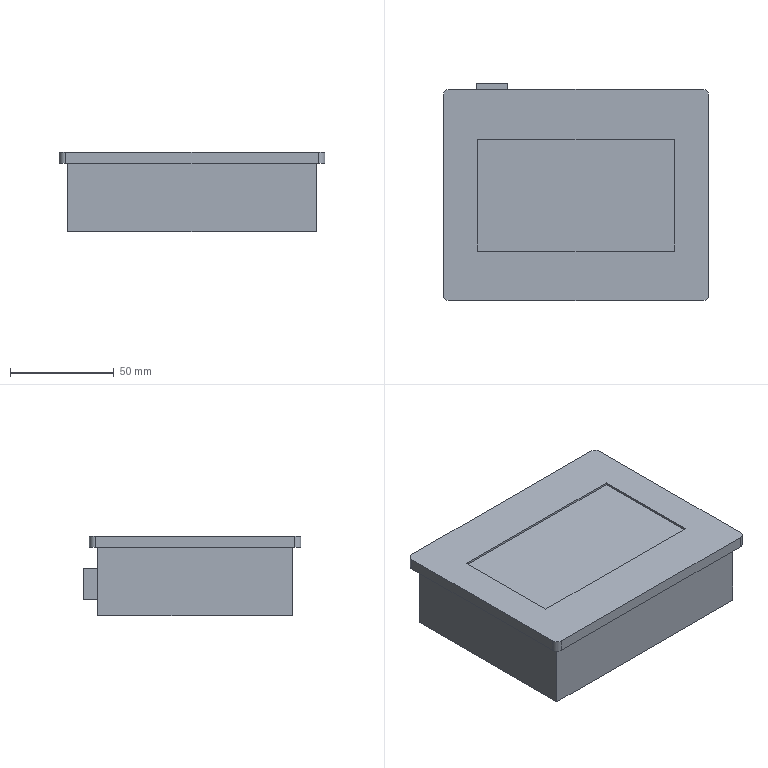Part | SolidWorks | features ICE 4, Extrusion 1, Fillet 1 | 2 solids | 31 faces | box 128 x 105 x 38.5 mm | volume 442026 mm3 | plane 27 | cylinder 4 | commonest cylinder face diameters 6 x4
STEP:
#1=CARTESIAN_POINT('',(-60.,47.,0.));
#2=VERTEX_POINT('',#1);
#3=CARTESIAN_POINT('',(60.,47.,0.));
#4=VERTEX_POINT('',#3);
#5=CARTESIAN_POINT('',(-60.,47.,0.));
#6=DIRECTION('',(1.,0.,0.));
#7=VECTOR('',#6,1000.);
#8=LINE('',#5,#7);
#9=EDGE_CURVE('',#2,#4,#8,.T.);
#10=ORIENTED_EDGE('',*,*,#9,.T.);
#11=CARTESIAN_POINT('',(60.,47.,-33.));
#12=VERTEX_POINT('',#11);
#13=CARTESIAN_POINT('',(60.,47.,-33.));
#14=DIRECTION('',(0.,0.,1.));
#15=VECTOR('',#14,1000.);
#16=LINE('',#13,#15);
#17=EDGE_CURVE('',#12,#4,#16,.T.);
#18=ORIENTED_EDGE('',*,*,#17,.F.);
#19=CARTESIAN_POINT('',(-60.,47.,-33.));
#20=VERTEX_POINT('',#19);
#21=CARTESIAN_POINT('',(-60.,47.,-33.));
#22=DIRECTION('',(1.,0.,0.));
#23=VECTOR('',#22,1000.);
#24=LINE('',#21,#23);
#25=EDGE_CURVE('',#20,#12,#24,.T.);
#26=ORIENTED_EDGE('',*,*,#25,.F.);
#27=CARTESIAN_POINT('',(-60.,47.,-33.));
#28=DIRECTION('',(0.,0.,1.));
#29=VECTOR('',#28,1000.);
#30=LINE('',#27,#29);
#31=EDGE_CURVE('',#20,#2,#30,.T.);
#32=ORIENTED_EDGE('',*,*,#31,.T.);
#33=EDGE_LOOP('',(#10,#18,#26,#32));
#34=FACE_OUTER_BOUND('',#33,.T.);
#35=CARTESIAN_POINT('',(-48.,47.,-25.));
#36=VERTEX_POINT('',#35);
#37=CARTESIAN_POINT('',(-48.,47.,-10.));
#38=VERTEX_POINT('',#37);
#39=CARTESIAN_POINT('',(-48.,47.,-25.));
#40=DIRECTION('',(0.,0.,1.));
#41=VECTOR('',#40,1000.);
#42=LINE('',#39,#41);
#43=EDGE_CURVE('',#36,#38,#42,.T.);
#44=ORIENTED_EDGE('',*,*,#43,.F.);
#45=CARTESIAN_POINT('',(-33.,47.,-25.));
#46=VERTEX_POINT('',#45);
#47=CARTESIAN_POINT('',(-48.,47.,-25.));
#48=DIRECTION('',(-1.,0.,0.));
#49=VECTOR('',#48,1000.);
#50=LINE('',#47,#49);
#51=EDGE_CURVE('',#46,#36,#50,.T.);
#52=ORIENTED_EDGE('',*,*,#51,.F.);
#53=CARTESIAN_POINT('',(-33.,47.,-10.));
#54=VERTEX_POINT('',#53);
#55=CARTESIAN_POINT('',(-33.,47.,-25.));
#56=DIRECTION('',(0.,0.,-1.));
#57=VECTOR('',#56,1000.);
#58=LINE('',#55,#57);
#59=EDGE_CURVE('',#54,#46,#58,.T.);
#60=ORIENTED_EDGE('',*,*,#59,.F.);
#61=CARTESIAN_POINT('',(-48.,47.,-10.));
#62=DIRECTION('',(1.,0.,0.));
#63=VECTOR('',#62,1000.);
#64=LINE('',#61,#63);
#65=EDGE_CURVE('',#38,#54,#64,.T.);
#66=ORIENTED_EDGE('',*,*,#65,.F.);
#67=EDGE_LOOP('',(#44,#52,#60,#66));
#68=FACE_BOUND('',#67,.T.);
#69=CARTESIAN_POINT('',(-60.,47.,-33.));
#70=DIRECTION('',(0.,-1.,0.));
#71=DIRECTION('',(1.,0.,0.));
#72=AXIS2_PLACEMENT_3D('',#69,#70,#71);
#73=PLANE('',#72);
#74=ADVANCED_FACE('',(#34,#68),#73,.F.);
#75=CARTESIAN_POINT('',(-64.,48.,0.));
#76=VERTEX_POINT('',#75);
#77=CARTESIAN_POINT('',(-64.,-48.,0.));
#78=VERTEX_POINT('',#77);
#79=CARTESIAN_POINT('',(-64.,-51.,0.));
#80=DIRECTION('',(0.,-1.,0.));
#81=VECTOR('',#80,1000.);
#82=LINE('',#79,#81);
#83=EDGE_CURVE('',#76,#78,#82,.T.);
#84=ORIENTED_EDGE('',*,*,#83,.F.);
#85=CARTESIAN_POINT('',(-61.,51.,0.));
#86=VERTEX_POINT('',#85);
#87=CARTESIAN_POINT('',(-61.,48.,0.));
#88=DIRECTION('',(0.,0.,-1.));
#89=DIRECTION('',(1.,0.,0.));
#90=AXIS2_PLACEMENT_3D('',#87,#88,#89);
#91=CIRCLE('',#90,3.);
#92=EDGE_CURVE('',#76,#86,#91,.T.);
#93=ORIENTED_EDGE('',*,*,#92,.T.);
#94=CARTESIAN_POINT('',(61.,51.,0.));
#95=VERTEX_POINT('',#94);
#96=CARTESIAN_POINT('',(64.,51.,0.));
#97=DIRECTION('',(-1.,0.,0.));
#98=VECTOR('',#97,1000.);
#99=LINE('',#96,#98);
#100=EDGE_CURVE('',#95,#86,#99,.T.);
#101=ORIENTED_EDGE('',*,*,#100,.F.);
#102=CARTESIAN_POINT('',(64.,48.,0.));
#103=VERTEX_POINT('',#102);
#104=CARTESIAN_POINT('',(61.,48.,0.));
#105=DIRECTION('',(0.,0.,-1.));
#106=DIRECTION('',(1.,0.,0.));
#107=AXIS2_PLACEMENT_3D('',#104,#105,#106);
#108=CIRCLE('',#107,3.);
#109=EDGE_CURVE('',#95,#103,#108,.T.);
#110=ORIENTED_EDGE('',*,*,#109,.T.);
#111=CARTESIAN_POINT('',(64.,-48.,0.));
#112=VERTEX_POINT('',#111);
#113=CARTESIAN_POINT('',(64.,-51.,0.));
#114=DIRECTION('',(0.,1.,0.));
#115=VECTOR('',#114,1000.);
#116=LINE('',#113,#115);
#117=EDGE_CURVE('',#112,#103,#116,.T.);
#118=ORIENTED_EDGE('',*,*,#117,.F.);
#119=CARTESIAN_POINT('',(61.,-51.,0.));
#120=VERTEX_POINT('',#119);
#121=CARTESIAN_POINT('',(61.,-48.,0.));
#122=DIRECTION('',(0.,0.,-1.));
#123=DIRECTION('',(1.,0.,0.));
#124=AXIS2_PLACEMENT_3D('',#121,#122,#123);
#125=CIRCLE('',#124,3.);
#126=EDGE_CURVE('',#112,#120,#125,.T.);
#127=ORIENTED_EDGE('',*,*,#126,.T.);
#128=CARTESIAN_POINT('',(-61.,-51.,0.));
#129=VERTEX_POINT('',#128);
#130=CARTESIAN_POINT('',(64.,-51.,0.));
#131=DIRECTION('',(1.,0.,0.));
#132=VECTOR('',#131,1000.);
#133=LINE('',#130,#132);
#134=EDGE_CURVE('',#129,#120,#133,.T.);
#135=ORIENTED_EDGE('',*,*,#134,.F.);
#136=CARTESIAN_POINT('',(-61.,-48.,0.));
#137=DIRECTION('',(0.,0.,-1.));
#138=DIRECTION('',(1.,0.,0.));
#139=AXIS2_PLACEMENT_3D('',#136,#137,#138);
#140=CIRCLE('',#139,3.);
#141=EDGE_CURVE('',#129,#78,#140,.T.);
#142=ORIENTED_EDGE('',*,*,#141,.T.);
#143=EDGE_LOOP('',(#84,#93,#101,#110,#118,#127,#135,#142));
#144=FACE_OUTER_BOUND('',#143,.T.);
#145=CARTESIAN_POINT('',(60.,-47.,0.));
#146=VERTEX_POINT('',#145);
#147=CARTESIAN_POINT('',(60.,-47.,0.));
#148=DIRECTION('',(0.,-1.,0.));
#149=VECTOR('',#148,1000.);
#150=LINE('',#147,#149);
#151=EDGE_CURVE('',#4,#146,#150,.T.);
#152=ORIENTED_EDGE('',*,*,#151,.F.);
#153=ORIENTED_EDGE('',*,*,#9,.F.);
#154=CARTESIAN_POINT('',(-60.,-47.,0.));
#155=VERTEX_POINT('',#154);
#156=CARTESIAN_POINT('',(-60.,-47.,0.));
#157=DIRECTION('',(0.,1.,0.));
#158=VECTOR('',#157,1000.);
#159=LINE('',#156,#158);
#160=EDGE_CURVE('',#155,#2,#159,.T.);
#161=ORIENTED_EDGE('',*,*,#160,.F.);
#162=CARTESIAN_POINT('',(-60.,-47.,0.));
#163=DIRECTION('',(-1.,0.,0.));
#164=VECTOR('',#163,1000.);
#165=LINE('',#162,#164);
#166=EDGE_CURVE('',#146,#155,#165,.T.);
#167=ORIENTED_EDGE('',*,*,#166,.F.);
#168=EDGE_LOOP('',(#152,#153,#161,#167));
#169=FACE_BOUND('',#168,.T.);
#170=CARTESIAN_POINT('',(0.,0.,0.));
#171=DIRECTION('',(0.,0.,1.));
#172=DIRECTION('',(1.,0.,0.));
#173=AXIS2_PLACEMENT_3D('',#170,#171,#172);
#174=PLANE('',#173);
#175=ADVANCED_FACE('',(#144,#169),#174,.F.);
#176=CARTESIAN_POINT('',(-64.,48.,5.5));
#177=VERTEX_POINT('',#176);
#178=CARTESIAN_POINT('',(-64.,-48.,5.5));
#179=VERTEX_POINT('',#178);
#180=CARTESIAN_POINT('',(-64.,-51.,5.5));
#181=DIRECTION('',(0.,-1.,0.));
#182=VECTOR('',#181,1000.);
#183=LINE('',#180,#182);
#184=EDGE_CURVE('',#177,#179,#183,.T.);
#185=ORIENTED_EDGE('',*,*,#184,.F.);
#186=CARTESIAN_POINT('',(-64.,48.,5.5));
#187=DIRECTION('',(0.,0.,-1.));
#188=VECTOR('',#187,1000.);
#189=LINE('',#186,#188);
#190=EDGE_CURVE('',#177,#76,#189,.T.);
#191=ORIENTED_EDGE('',*,*,#190,.T.);
#192=ORIENTED_EDGE('',*,*,#83,.T.);
#193=CARTESIAN_POINT('',(-64.,-48.,5.5));
#194=DIRECTION('',(0.,0.,1.));
#195=VECTOR('',#194,1000.);
#196=LINE('',#193,#195);
#197=EDGE_CURVE('',#78,#179,#196,.T.);
#198=ORIENTED_EDGE('',*,*,#197,.T.);
#199=EDGE_LOOP('',(#185,#191,#192,#198));
#200=FACE_OUTER_BOUND('',#199,.T.);
#201=CARTESIAN_POINT('',(-64.,-51.,5.5));
#202=DIRECTION('',(1.,0.,0.));
#203=DIRECTION('',(0.,0.,-1.));
#204=AXIS2_PLACEMENT_3D('',#201,#202,#203);
#205=PLANE('',#204);
#206=ADVANCED_FACE('',(#200),#205,.F.);
#207=ORIENTED_EDGE('',*,*,#134,.T.);
#208=CARTESIAN_POINT('',(61.,-51.,5.5));
#209=VERTEX_POINT('',#208);
#210=CARTESIAN_POINT('',(61.,-51.,5.5));
#211=DIRECTION('',(0.,0.,1.));
#212=VECTOR('',#211,1000.);
#213=LINE('',#210,#212);
#214=EDGE_CURVE('',#120,#209,#213,.T.);
#215=ORIENTED_EDGE('',*,*,#214,.T.);
#216=CARTESIAN_POINT('',(-61.,-51.,5.5));
#217=VERTEX_POINT('',#216);
#218=CARTESIAN_POINT('',(64.,-51.,5.5));
#219=DIRECTION('',(1.,0.,0.));
#220=VECTOR('',#219,1000.);
#221=LINE('',#218,#220);
#222=EDGE_CURVE('',#217,#209,#221,.T.);
#223=ORIENTED_EDGE('',*,*,#222,.F.);
#224=CARTESIAN_POINT('',(-61.,-51.,5.5));
#225=DIRECTION('',(0.,0.,-1.));
#226=VECTOR('',#225,1000.);
#227=LINE('',#224,#226);
#228=EDGE_CURVE('',#217,#129,#227,.T.);
#229=ORIENTED_EDGE('',*,*,#228,.T.);
#230=EDGE_LOOP('',(#207,#215,#223,#229));
#231=FACE_OUTER_BOUND('',#230,.T.);
#232=CARTESIAN_POINT('',(64.,-51.,5.5));
#233=DIRECTION('',(0.,1.,0.));
#234=DIRECTION('',(-1.,0.,0.));
#235=AXIS2_PLACEMENT_3D('',#232,#233,#234);
#236=PLANE('',#235);
#237=ADVANCED_FACE('',(#231),#236,.F.);
#238=ORIENTED_EDGE('',*,*,#117,.T.);
#239=CARTESIAN_POINT('',(64.,48.,5.5));
#240=VERTEX_POINT('',#239);
#241=CARTESIAN_POINT('',(64.,48.,5.5));
#242=DIRECTION('',(0.,0.,1.));
#243=VECTOR('',#242,1000.);
#244=LINE('',#241,#243);
#245=EDGE_CURVE('',#103,#240,#244,.T.);
#246=ORIENTED_EDGE('',*,*,#245,.T.);
#247=CARTESIAN_POINT('',(64.,-48.,5.5));
#248=VERTEX_POINT('',#247);
#249=CARTESIAN_POINT('',(64.,-51.,5.5));
#250=DIRECTION('',(0.,1.,0.));
#251=VECTOR('',#250,1000.);
#252=LINE('',#249,#251);
#253=EDGE_CURVE('',#248,#240,#252,.T.);
#254=ORIENTED_EDGE('',*,*,#253,.F.);
#255=CARTESIAN_POINT('',(64.,-48.,5.5));
#256=DIRECTION('',(0.,0.,-1.));
#257=VECTOR('',#256,1000.);
#258=LINE('',#255,#257);
#259=EDGE_CURVE('',#248,#112,#258,.T.);
#260=ORIENTED_EDGE('',*,*,#259,.T.);
#261=EDGE_LOOP('',(#238,#246,#254,#260));
#262=FACE_OUTER_BOUND('',#261,.T.);
#263=CARTESIAN_POINT('',(64.,-51.,5.5));
#264=DIRECTION('',(-1.,0.,0.));
#265=DIRECTION('',(0.,0.,1.));
#266=AXIS2_PLACEMENT_3D('',#263,#264,#265);
#267=PLANE('',#266);
#268=ADVANCED_FACE('',(#262),#267,.F.);
#269=ORIENTED_EDGE('',*,*,#100,.T.);
#270=CARTESIAN_POINT('',(-61.,51.,5.5));
#271=VERTEX_POINT('',#270);
#272=CARTESIAN_POINT('',(-61.,51.,5.5));
#273=DIRECTION('',(0.,0.,1.));
#274=VECTOR('',#273,1000.);
#275=LINE('',#272,#274);
#276=EDGE_CURVE('',#86,#271,#275,.T.);
#277=ORIENTED_EDGE('',*,*,#276,.T.);
#278=CARTESIAN_POINT('',(61.,51.,5.5));
#279=VERTEX_POINT('',#278);
#280=CARTESIAN_POINT('',(64.,51.,5.5));
#281=DIRECTION('',(-1.,0.,0.));
#282=VECTOR('',#281,1000.);
#283=LINE('',#280,#282);
#284=EDGE_CURVE('',#279,#271,#283,.T.);
#285=ORIENTED_EDGE('',*,*,#284,.F.);
#286=CARTESIAN_POINT('',(61.,51.,5.5));
#287=DIRECTION('',(0.,0.,-1.));
#288=VECTOR('',#287,1000.);
#289=LINE('',#286,#288);
#290=EDGE_CURVE('',#279,#95,#289,.T.);
#291=ORIENTED_EDGE('',*,*,#290,.T.);
#292=EDGE_LOOP('',(#269,#277,#285,#291));
#293=FACE_OUTER_BOUND('',#292,.T.);
#294=CARTESIAN_POINT('',(64.,51.,5.5));
#295=DIRECTION('',(0.,-1.,0.));
#296=DIRECTION('',(1.,0.,0.));
#297=AXIS2_PLACEMENT_3D('',#294,#295,#296);
#298=PLANE('',#297);
#299=ADVANCED_FACE('',(#293),#298,.F.);
#300=CARTESIAN_POINT('',(-47.5,27.,5.5));
#301=VERTEX_POINT('',#300);
#302=CARTESIAN_POINT('',(-47.5,-27.,5.5));
#303=VERTEX_POINT('',#302);
#304=CARTESIAN_POINT('',(-47.5,-27.,5.5));
#305=DIRECTION('',(0.,-1.,0.));
#306=VECTOR('',#305,1000.);
#307=LINE('',#304,#306);
#308=EDGE_CURVE('',#301,#303,#307,.T.);
#309=ORIENTED_EDGE('',*,*,#308,.F.);
#310=CARTESIAN_POINT('',(47.5,27.,5.5));
#311=VERTEX_POINT('',#310);
#312=CARTESIAN_POINT('',(47.5,27.,5.5));
#313=DIRECTION('',(-1.,0.,0.));
#314=VECTOR('',#313,1000.);
#315=LINE('',#312,#314);
#316=EDGE_CURVE('',#311,#301,#315,.T.);
#317=ORIENTED_EDGE('',*,*,#316,.F.);
#318=CARTESIAN_POINT('',(47.5,-27.,5.5));
#319=VERTEX_POINT('',#318);
#320=CARTESIAN_POINT('',(47.5,-27.,5.5));
#321=DIRECTION('',(0.,1.,0.));
#322=VECTOR('',#321,1000.);
#323=LINE('',#320,#322);
#324=EDGE_CURVE('',#319,#311,#323,.T.);
#325=ORIENTED_EDGE('',*,*,#324,.F.);
#326=CARTESIAN_POINT('',(47.5,-27.,5.5));
#327=DIRECTION('',(1.,0.,0.));
#328=VECTOR('',#327,1000.);
#329=LINE('',#326,#328);
#330=EDGE_CURVE('',#303,#319,#329,.T.);
#331=ORIENTED_EDGE('',*,*,#330,.F.);
#332=EDGE_LOOP('',(#309,#317,#325,#331));
#333=FACE_BOUND('',#332,.T.);
#334=ORIENTED_EDGE('',*,*,#284,.T.);
#335=CARTESIAN_POINT('',(-61.,48.,5.5));
#336=DIRECTION('',(0.,0.,1.));
#337=DIRECTION('',(1.,0.,0.));
#338=AXIS2_PLACEMENT_3D('',#335,#336,#337);
#339=CIRCLE('',#338,3.);
#340=EDGE_CURVE('',#271,#177,#339,.T.);
#341=ORIENTED_EDGE('',*,*,#340,.T.);
#342=ORIENTED_EDGE('',*,*,#184,.T.);
#343=CARTESIAN_POINT('',(-61.,-48.,5.5));
#344=DIRECTION('',(0.,0.,1.));
#345=DIRECTION('',(1.,0.,0.));
#346=AXIS2_PLACEMENT_3D('',#343,#344,#345);
#347=CIRCLE('',#346,3.);
#348=EDGE_CURVE('',#179,#217,#347,.T.);
#349=ORIENTED_EDGE('',*,*,#348,.T.);
#350=ORIENTED_EDGE('',*,*,#222,.T.);
#351=CARTESIAN_POINT('',(61.,-48.,5.5));
#352=DIRECTION('',(0.,0.,1.));
#353=DIRECTION('',(1.,0.,0.));
#354=AXIS2_PLACEMENT_3D('',#351,#352,#353);
#355=CIRCLE('',#354,3.);
#356=EDGE_CURVE('',#209,#248,#355,.T.);
#357=ORIENTED_EDGE('',*,*,#356,.T.);
#358=ORIENTED_EDGE('',*,*,#253,.T.);
#359=CARTESIAN_POINT('',(61.,48.,5.5));
#360=DIRECTION('',(0.,0.,1.));
#361=DIRECTION('',(1.,0.,0.));
#362=AXIS2_PLACEMENT_3D('',#359,#360,#361);
#363=CIRCLE('',#362,3.);
#364=EDGE_CURVE('',#240,#279,#363,.T.);
#365=ORIENTED_EDGE('',*,*,#364,.T.);
#366=EDGE_LOOP('',(#334,#341,#342,#349,#350,#357,#358,#365));
#367=FACE_OUTER_BOUND('',#366,.T.);
#368=CARTESIAN_POINT('',(0.,0.,5.5));
#369=DIRECTION('',(0.,0.,1.));
#370=DIRECTION('',(1.,0.,0.));
#371=AXIS2_PLACEMENT_3D('',#368,#369,#370);
#372=PLANE('',#371);
#373=ADVANCED_FACE('',(#333,#367),#372,.T.);
#374=ORIENTED_EDGE('',*,*,#308,.T.);
#375=CARTESIAN_POINT('',(-47.5,-27.,4.5));
#376=VERTEX_POINT('',#375);
#377=CARTESIAN_POINT('',(-47.5,-27.,4.5));
#378=DIRECTION('',(0.,0.,1.));
#379=VECTOR('',#378,1000.);
#380=LINE('',#377,#379);
#381=EDGE_CURVE('',#376,#303,#380,.T.);
#382=ORIENTED_EDGE('',*,*,#381,.F.);
#383=CARTESIAN_POINT('',(-47.5,27.,4.5));
#384=VERTEX_POINT('',#383);
#385=CARTESIAN_POINT('',(-47.5,-27.,4.5));
#386=DIRECTION('',(0.,-1.,0.));
#387=VECTOR('',#386,1000.);
#388=LINE('',#385,#387);
#389=EDGE_CURVE('',#384,#376,#388,.T.);
#390=ORIENTED_EDGE('',*,*,#389,.F.);
#391=CARTESIAN_POINT('',(-47.5,27.,4.5));
#392=DIRECTION('',(0.,0.,1.));
#393=VECTOR('',#392,1000.);
#394=LINE('',#391,#393);
#395=EDGE_CURVE('',#384,#301,#394,.T.);
#396=ORIENTED_EDGE('',*,*,#395,.T.);
#397=EDGE_LOOP('',(#374,#382,#390,#396));
#398=FACE_OUTER_BOUND('',#397,.T.);
#399=CARTESIAN_POINT('',(-47.5,-27.,4.5));
#400=DIRECTION('',(-1.,0.,0.));
#401=DIRECTION('',(0.,0.,1.));
#402=AXIS2_PLACEMENT_3D('',#399,#400,#401);
#403=PLANE('',#402);
#404=ADVANCED_FACE('',(#398),#403,.F.);
#405=ORIENTED_EDGE('',*,*,#316,.T.);
#406=ORIENTED_EDGE('',*,*,#395,.F.);
#407=CARTESIAN_POINT('',(47.5,27.,4.5));
#408=VERTEX_POINT('',#407);
#409=CARTESIAN_POINT('',(47.5,27.,4.5));
#410=DIRECTION('',(-1.,0.,0.));
#411=VECTOR('',#410,1000.);
#412=LINE('',#409,#411);
#413=EDGE_CURVE('',#408,#384,#412,.T.);
#414=ORIENTED_EDGE('',*,*,#413,.F.);
#415=CARTESIAN_POINT('',(47.5,27.,4.5));
#416=DIRECTION('',(0.,0.,1.));
#417=VECTOR('',#416,1000.);
#418=LINE('',#415,#417);
#419=EDGE_CURVE('',#408,#311,#418,.T.);
#420=ORIENTED_EDGE('',*,*,#419,.T.);
#421=EDGE_LOOP('',(#405,#406,#414,#420));
#422=FACE_OUTER_BOUND('',#421,.T.);
#423=CARTESIAN_POINT('',(47.5,27.,4.5));
#424=DIRECTION('',(0.,1.,0.));
#425=DIRECTION('',(-1.,0.,0.));
#426=AXIS2_PLACEMENT_3D('',#423,#424,#425);
#427=PLANE('',#426);
#428=ADVANCED_FACE('',(#422),#427,.F.);
#429=ORIENTED_EDGE('',*,*,#324,.T.);
#430=ORIENTED_EDGE('',*,*,#419,.F.);
#431=CARTESIAN_POINT('',(47.5,-27.,4.5));
#432=VERTEX_POINT('',#431);
#433=CARTESIAN_POINT('',(47.5,-27.,4.5));
#434=DIRECTION('',(0.,1.,0.));
#435=VECTOR('',#434,1000.);
#436=LINE('',#433,#435);
#437=EDGE_CURVE('',#432,#408,#436,.T.);
#438=ORIENTED_EDGE('',*,*,#437,.F.);
#439=CARTESIAN_POINT('',(47.5,-27.,4.5));
#440=DIRECTION('',(0.,0.,1.));
#441=VECTOR('',#440,1000.);
#442=LINE('',#439,#441);
#443=EDGE_CURVE('',#432,#319,#442,.T.);
#444=ORIENTED_EDGE('',*,*,#443,.T.);
#445=EDGE_LOOP('',(#429,#430,#438,#444));
#446=FACE_OUTER_BOUND('',#445,.T.);
#447=CARTESIAN_POINT('',(47.5,-27.,4.5));
#448=DIRECTION('',(1.,0.,0.));
#449=DIRECTION('',(0.,0.,-1.));
#450=AXIS2_PLACEMENT_3D('',#447,#448,#449);
#451=PLANE('',#450);
#452=ADVANCED_FACE('',(#446),#451,.F.);
#453=ORIENTED_EDGE('',*,*,#330,.T.);
#454=ORIENTED_EDGE('',*,*,#443,.F.);
#455=CARTESIAN_POINT('',(47.5,-27.,4.5));
#456=DIRECTION('',(1.,0.,0.));
#457=VECTOR('',#456,1000.);
#458=LINE('',#455,#457);
#459=EDGE_CURVE('',#376,#432,#458,.T.);
#460=ORIENTED_EDGE('',*,*,#459,.F.);
#461=ORIENTED_EDGE('',*,*,#381,.T.);
#462=EDGE_LOOP('',(#453,#454,#460,#461));
#463=FACE_OUTER_BOUND('',#462,.T.);
#464=CARTESIAN_POINT('',(47.5,-27.,4.5));
#465=DIRECTION('',(0.,-1.,0.));
#466=DIRECTION('',(1.,0.,0.));
#467=AXIS2_PLACEMENT_3D('',#464,#465,#466);
#468=PLANE('',#467);
#469=ADVANCED_FACE('',(#463),#468,.F.);
#470=ORIENTED_EDGE('',*,*,#389,.T.);
#471=ORIENTED_EDGE('',*,*,#459,.T.);
#472=ORIENTED_EDGE('',*,*,#437,.T.);
#473=ORIENTED_EDGE('',*,*,#413,.T.);
#474=EDGE_LOOP('',(#470,#471,#472,#473));
#475=FACE_OUTER_BOUND('',#474,.T.);
#476=CARTESIAN_POINT('',(0.,0.,4.5));
#477=DIRECTION('',(0.,0.,1.));
#478=DIRECTION('',(1.,0.,0.));
#479=AXIS2_PLACEMENT_3D('',#476,#477,#478);
#480=PLANE('',#479);
#481=ADVANCED_FACE('',(#475),#480,.T.);
#482=ORIENTED_EDGE('',*,*,#151,.T.);
#483=CARTESIAN_POINT('',(60.,-47.,-33.));
#484=VERTEX_POINT('',#483);
#485=CARTESIAN_POINT('',(60.,-47.,-33.));
#486=DIRECTION('',(0.,0.,1.));
#487=VECTOR('',#486,1000.);
#488=LINE('',#485,#487);
#489=EDGE_CURVE('',#484,#146,#488,.T.);
#490=ORIENTED_EDGE('',*,*,#489,.F.);
#491=CARTESIAN_POINT('',(60.,-47.,-33.));
#492=DIRECTION('',(0.,-1.,0.));
#493=VECTOR('',#492,1000.);
#494=LINE('',#491,#493);
#495=EDGE_CURVE('',#12,#484,#494,.T.);
#496=ORIENTED_EDGE('',*,*,#495,.F.);
#497=ORIENTED_EDGE('',*,*,#17,.T.);
#498=EDGE_LOOP('',(#482,#490,#496,#497));
#499=FACE_OUTER_BOUND('',#498,.T.);
#500=CARTESIAN_POINT('',(60.,-47.,-33.));
#501=DIRECTION('',(-1.,0.,0.));
#502=DIRECTION('',(0.,0.,1.));
#503=AXIS2_PLACEMENT_3D('',#500,#501,#502);
#504=PLANE('',#503);
#505=ADVANCED_FACE('',(#499),#504,.F.);
#506=ORIENTED_EDGE('',*,*,#166,.T.);
#507=CARTESIAN_POINT('',(-60.,-47.,-33.));
#508=VERTEX_POINT('',#507);
#509=CARTESIAN_POINT('',(-60.,-47.,-33.));
#510=DIRECTION('',(0.,0.,1.));
#511=VECTOR('',#510,1000.);
#512=LINE('',#509,#511);
#513=EDGE_CURVE('',#508,#155,#512,.T.);
#514=ORIENTED_EDGE('',*,*,#513,.F.);
#515=CARTESIAN_POINT('',(-60.,-47.,-33.));
#516=DIRECTION('',(-1.,0.,0.));
#517=VECTOR('',#516,1000.);
#518=LINE('',#515,#517);
#519=EDGE_CURVE('',#484,#508,#518,.T.);
#520=ORIENTED_EDGE('',*,*,#519,.F.);
#521=ORIENTED_EDGE('',*,*,#489,.T.);
#522=EDGE_LOOP('',(#506,#514,#520,#521));
#523=FACE_OUTER_BOUND('',#522,.T.);
#524=CARTESIAN_POINT('',(-60.,-47.,-33.));
#525=DIRECTION('',(0.,1.,0.));
#526=DIRECTION('',(-1.,0.,0.));
#527=AXIS2_PLACEMENT_3D('',#524,#525,#526);
#528=PLANE('',#527);
#529=ADVANCED_FACE('',(#523),#528,.F.);
#530=ORIENTED_EDGE('',*,*,#160,.T.);
#531=ORIENTED_EDGE('',*,*,#31,.F.);
#532=CARTESIAN_POINT('',(-60.,-47.,-33.));
#533=DIRECTION('',(0.,1.,0.));
#534=VECTOR('',#533,1000.);
#535=LINE('',#532,#534);
#536=EDGE_CURVE('',#508,#20,#535,.T.);
#537=ORIENTED_EDGE('',*,*,#536,.F.);
#538=ORIENTED_EDGE('',*,*,#513,.T.);
#539=EDGE_LOOP('',(#530,#531,#537,#538));
#540=FACE_OUTER_BOUND('',#539,.T.);
#541=CARTESIAN_POINT('',(-60.,-47.,-33.));
#542=DIRECTION('',(1.,0.,0.));
#543=DIRECTION('',(0.,0.,-1.));
#544=AXIS2_PLACEMENT_3D('',#541,#542,#543);
#545=PLANE('',#544);
#546=ADVANCED_FACE('',(#540),#545,.F.);
#547=ORIENTED_EDGE('',*,*,#495,.T.);
#548=ORIENTED_EDGE('',*,*,#519,.T.);
#549=ORIENTED_EDGE('',*,*,#536,.T.);
#550=ORIENTED_EDGE('',*,*,#25,.T.);
#551=EDGE_LOOP('',(#547,#548,#549,#550));
#552=FACE_OUTER_BOUND('',#551,.T.);
#553=CARTESIAN_POINT('',(0.,0.,-33.));
#554=DIRECTION('',(0.,0.,-1.));
#555=DIRECTION('',(-1.,0.,0.));
#556=AXIS2_PLACEMENT_3D('',#553,#554,#555);
#557=PLANE('',#556);
#558=ADVANCED_FACE('',(#552),#557,.T.);
#559=ORIENTED_EDGE('',*,*,#340,.F.);
#560=ORIENTED_EDGE('',*,*,#276,.F.);
#561=ORIENTED_EDGE('',*,*,#92,.F.);
#562=ORIENTED_EDGE('',*,*,#190,.F.);
#563=EDGE_LOOP('',(#559,#560,#561,#562));
#564=FACE_OUTER_BOUND('',#563,.T.);
#565=CARTESIAN_POINT('',(-61.,48.,5.5));
#566=DIRECTION('',(0.,0.,-1.));
#567=DIRECTION('',(-1.,0.,0.));
#568=AXIS2_PLACEMENT_3D('',#565,#566,#567);
#569=CYLINDRICAL_SURFACE('',#568,3.);
#570=ADVANCED_FACE('',(#564),#569,.T.);
#571=ORIENTED_EDGE('',*,*,#364,.F.);
#572=ORIENTED_EDGE('',*,*,#245,.F.);
#573=ORIENTED_EDGE('',*,*,#109,.F.);
#574=ORIENTED_EDGE('',*,*,#290,.F.);
#575=EDGE_LOOP('',(#571,#572,#573,#574));
#576=FACE_OUTER_BOUND('',#575,.T.);
#577=CARTESIAN_POINT('',(61.,48.,5.5));
#578=DIRECTION('',(0.,0.,-1.));
#579=DIRECTION('',(-1.,0.,0.));
#580=AXIS2_PLACEMENT_3D('',#577,#578,#579);
#581=CYLINDRICAL_SURFACE('',#580,3.);
#582=ADVANCED_FACE('',(#576),#581,.T.);
#583=ORIENTED_EDGE('',*,*,#356,.F.);
#584=ORIENTED_EDGE('',*,*,#214,.F.);
#585=ORIENTED_EDGE('',*,*,#126,.F.);
#586=ORIENTED_EDGE('',*,*,#259,.F.);
#587=EDGE_LOOP('',(#583,#584,#585,#586));
#588=FACE_OUTER_BOUND('',#587,.T.);
#589=CARTESIAN_POINT('',(61.,-48.,5.5));
#590=DIRECTION('',(0.,0.,-1.));
#591=DIRECTION('',(-1.,0.,0.));
#592=AXIS2_PLACEMENT_3D('',#589,#590,#591);
#593=CYLINDRICAL_SURFACE('',#592,3.);
#594=ADVANCED_FACE('',(#588),#593,.T.);
#595=ORIENTED_EDGE('',*,*,#348,.F.);
#596=ORIENTED_EDGE('',*,*,#197,.F.);
#597=ORIENTED_EDGE('',*,*,#141,.F.);
#598=ORIENTED_EDGE('',*,*,#228,.F.);
#599=EDGE_LOOP('',(#595,#596,#597,#598));
#600=FACE_OUTER_BOUND('',#599,.T.);
#601=CARTESIAN_POINT('',(-61.,-48.,5.5));
#602=DIRECTION('',(0.,0.,-1.));
#603=DIRECTION('',(-1.,0.,0.));
#604=AXIS2_PLACEMENT_3D('',#601,#602,#603);
#605=CYLINDRICAL_SURFACE('',#604,3.);
#606=ADVANCED_FACE('',(#600),#605,.T.);
#607=ORIENTED_EDGE('',*,*,#43,.T.);
#608=CARTESIAN_POINT('',(-48.,54.,-10.));
#609=VERTEX_POINT('',#608);
#610=CARTESIAN_POINT('',(-48.,54.,-10.));
#611=DIRECTION('',(0.,-1.,0.));
#612=VECTOR('',#611,1000.);
#613=LINE('',#610,#612);
#614=EDGE_CURVE('',#609,#38,#613,.T.);
#615=ORIENTED_EDGE('',*,*,#614,.F.);
#616=CARTESIAN_POINT('',(-48.,54.,-25.));
#617=VERTEX_POINT('',#616);
#618=CARTESIAN_POINT('',(-48.,54.,-25.));
#619=DIRECTION('',(0.,0.,1.));
#620=VECTOR('',#619,1000.);
#621=LINE('',#618,#620);
#622=EDGE_CURVE('',#617,#609,#621,.T.);
#623=ORIENTED_EDGE('',*,*,#622,.F.);
#624=CARTESIAN_POINT('',(-48.,54.,-25.));
#625=DIRECTION('',(0.,-1.,0.));
#626=VECTOR('',#625,1000.);
#627=LINE('',#624,#626);
#628=EDGE_CURVE('',#617,#36,#627,.T.);
#629=ORIENTED_EDGE('',*,*,#628,.T.);
#630=EDGE_LOOP('',(#607,#615,#623,#629));
#631=FACE_OUTER_BOUND('',#630,.T.);
#632=CARTESIAN_POINT('',(-48.,54.,-25.));
#633=DIRECTION('',(1.,0.,0.));
#634=DIRECTION('',(0.,1.,0.));
#635=AXIS2_PLACEMENT_3D('',#632,#633,#634);
#636=PLANE('',#635);
#637=ADVANCED_FACE('',(#631),#636,.F.);
#638=ORIENTED_EDGE('',*,*,#65,.T.);
#639=CARTESIAN_POINT('',(-33.,54.,-10.));
#640=VERTEX_POINT('',#639);
#641=CARTESIAN_POINT('',(-33.,54.,-10.));
#642=DIRECTION('',(0.,-1.,0.));
#643=VECTOR('',#642,1000.);
#644=LINE('',#641,#643);
#645=EDGE_CURVE('',#640,#54,#644,.T.);
#646=ORIENTED_EDGE('',*,*,#645,.F.);
#647=CARTESIAN_POINT('',(-48.,54.,-10.));
#648=DIRECTION('',(1.,0.,0.));
#649=VECTOR('',#648,1000.);
#650=LINE('',#647,#649);
#651=EDGE_CURVE('',#609,#640,#650,.T.);
#652=ORIENTED_EDGE('',*,*,#651,.F.);
#653=ORIENTED_EDGE('',*,*,#614,.T.);
#654=EDGE_LOOP('',(#638,#646,#652,#653));
#655=FACE_OUTER_BOUND('',#654,.T.);
#656=CARTESIAN_POINT('',(-48.,54.,-10.));
#657=DIRECTION('',(0.,0.,-1.));
#658=DIRECTION('',(-1.,0.,0.));
#659=AXIS2_PLACEMENT_3D('',#656,#657,#658);
#660=PLANE('',#659);
#661=ADVANCED_FACE('',(#655),#660,.F.);
#662=ORIENTED_EDGE('',*,*,#59,.T.);
#663=CARTESIAN_POINT('',(-33.,54.,-25.));
#664=VERTEX_POINT('',#663);
#665=CARTESIAN_POINT('',(-33.,54.,-25.));
#666=DIRECTION('',(0.,-1.,0.));
#667=VECTOR('',#666,1000.);
#668=LINE('',#665,#667);
#669=EDGE_CURVE('',#664,#46,#668,.T.);
#670=ORIENTED_EDGE('',*,*,#669,.F.);
#671=CARTESIAN_POINT('',(-33.,54.,-25.));
#672=DIRECTION('',(0.,0.,-1.));
#673=VECTOR('',#672,1000.);
#674=LINE('',#671,#673);
#675=EDGE_CURVE('',#640,#664,#674,.T.);
#676=ORIENTED_EDGE('',*,*,#675,.F.);
#677=ORIENTED_EDGE('',*,*,#645,.T.);
#678=EDGE_LOOP('',(#662,#670,#676,#677));
#679=FACE_OUTER_BOUND('',#678,.T.);
#680=CARTESIAN_POINT('',(-33.,54.,-25.));
#681=DIRECTION('',(-1.,0.,0.));
#682=DIRECTION('',(0.,0.,1.));
#683=AXIS2_PLACEMENT_3D('',#680,#681,#682);
#684=PLANE('',#683);
#685=ADVANCED_FACE('',(#679),#684,.F.);
#686=ORIENTED_EDGE('',*,*,#51,.T.);
#687=ORIENTED_EDGE('',*,*,#628,.F.);
#688=CARTESIAN_POINT('',(-48.,54.,-25.));
#689=DIRECTION('',(-1.,0.,0.));
#690=VECTOR('',#689,1000.);
#691=LINE('',#688,#690);
#692=EDGE_CURVE('',#664,#617,#691,.T.);
#693=ORIENTED_EDGE('',*,*,#692,.F.);
#694=ORIENTED_EDGE('',*,*,#669,.T.);
#695=EDGE_LOOP('',(#686,#687,#693,#694));
#696=FACE_OUTER_BOUND('',#695,.T.);
#697=CARTESIAN_POINT('',(-48.,54.,-25.));
#698=DIRECTION('',(0.,0.,1.));
#699=DIRECTION('',(1.,0.,0.));
#700=AXIS2_PLACEMENT_3D('',#697,#698,#699);
#701=PLANE('',#700);
#702=ADVANCED_FACE('',(#696),#701,.F.);
#703=ORIENTED_EDGE('',*,*,#622,.T.);
#704=ORIENTED_EDGE('',*,*,#651,.T.);
#705=ORIENTED_EDGE('',*,*,#675,.T.);
#706=ORIENTED_EDGE('',*,*,#692,.T.);
#707=EDGE_LOOP('',(#703,#704,#705,#706));
#708=FACE_OUTER_BOUND('',#707,.T.);
#709=CARTESIAN_POINT('',(0.,54.,0.));
#710=DIRECTION('',(0.,1.,0.));
#711=DIRECTION('',(0.,0.,1.));
#712=AXIS2_PLACEMENT_3D('',#709,#710,#711);
#713=PLANE('',#712);
#714=ADVANCED_FACE('',(#708),#713,.T.);
#715=CLOSED_SHELL('',(#74,#175,#206,#237,#268,#299,#373,#404,#428,#452,#469,#481,#505,#529,#546,#558,#570,#582,#594,#606,#637,#661,#685,#702,#714));
#716=MANIFOLD_SOLID_BREP('',#715);
#717=CARTESIAN_POINT('',(-33.,47.,-25.));
#718=VERTEX_POINT('',#717);
#719=CARTESIAN_POINT('',(-33.,47.,-10.));
#720=VERTEX_POINT('',#719);
#721=CARTESIAN_POINT('',(-33.,47.,-25.));
#722=DIRECTION('',(0.,0.,1.));
#723=VECTOR('',#722,1000.);
#724=LINE('',#721,#723);
#725=EDGE_CURVE('',#718,#720,#724,.T.);
#726=ORIENTED_EDGE('',*,*,#725,.T.);
#727=CARTESIAN_POINT('',(-33.,50.,-10.));
#728=VERTEX_POINT('',#727);
#729=CARTESIAN_POINT('',(-33.,50.,-10.));
#730=DIRECTION('',(0.,-1.,0.));
#731=VECTOR('',#730,1000.);
#732=LINE('',#729,#731);
#733=EDGE_CURVE('',#728,#720,#732,.T.);
#734=ORIENTED_EDGE('',*,*,#733,.F.);
#735=CARTESIAN_POINT('',(-33.,50.,-25.));
#736=VERTEX_POINT('',#735);
#737=CARTESIAN_POINT('',(-33.,50.,-25.));
#738=DIRECTION('',(0.,0.,1.));
#739=VECTOR('',#738,1000.);
#740=LINE('',#737,#739);
#741=EDGE_CURVE('',#736,#728,#740,.T.);
#742=ORIENTED_EDGE('',*,*,#741,.F.);
#743=CARTESIAN_POINT('',(-33.,50.,-25.));
#744=DIRECTION('',(0.,-1.,0.));
#745=VECTOR('',#744,1000.);
#746=LINE('',#743,#745);
#747=EDGE_CURVE('',#736,#718,#746,.T.);
#748=ORIENTED_EDGE('',*,*,#747,.T.);
#749=EDGE_LOOP('',(#726,#734,#742,#748));
#750=FACE_OUTER_BOUND('',#749,.T.);
#751=CARTESIAN_POINT('',(-33.,50.,-25.));
#752=DIRECTION('',(1.,0.,0.));
#753=DIRECTION('',(0.,0.,-1.));
#754=AXIS2_PLACEMENT_3D('',#751,#752,#753);
#755=PLANE('',#754);
#756=ADVANCED_FACE('',(#750),#755,.F.);
#757=CARTESIAN_POINT('',(2.,47.,-10.));
#758=VERTEX_POINT('',#757);
#759=CARTESIAN_POINT('',(-33.,47.,-10.));
#760=DIRECTION('',(1.,0.,0.));
#761=VECTOR('',#760,1000.);
#762=LINE('',#759,#761);
#763=EDGE_CURVE('',#720,#758,#762,.T.);
#764=ORIENTED_EDGE('',*,*,#763,.T.);
#765=CARTESIAN_POINT('',(2.,50.,-10.));
#766=VERTEX_POINT('',#765);
#767=CARTESIAN_POINT('',(2.,50.,-10.));
#768=DIRECTION('',(0.,-1.,0.));
#769=VECTOR('',#768,1000.);
#770=LINE('',#767,#769);
#771=EDGE_CURVE('',#766,#758,#770,.T.);
#772=ORIENTED_EDGE('',*,*,#771,.F.);
#773=CARTESIAN_POINT('',(-33.,50.,-10.));
#774=DIRECTION('',(1.,0.,0.));
#775=VECTOR('',#774,1000.);
#776=LINE('',#773,#775);
#777=EDGE_CURVE('',#728,#766,#776,.T.);
#778=ORIENTED_EDGE('',*,*,#777,.F.);
#779=ORIENTED_EDGE('',*,*,#733,.T.);
#780=EDGE_LOOP('',(#764,#772,#778,#779));
#781=FACE_OUTER_BOUND('',#780,.T.);
#782=CARTESIAN_POINT('',(-33.,50.,-10.));
#783=DIRECTION('',(0.,0.,-1.));
#784=DIRECTION('',(-1.,0.,0.));
#785=AXIS2_PLACEMENT_3D('',#782,#783,#784);
#786=PLANE('',#785);
#787=ADVANCED_FACE('',(#781),#786,.F.);
#788=CARTESIAN_POINT('',(2.,47.,-25.));
#789=VERTEX_POINT('',#788);
#790=CARTESIAN_POINT('',(2.,47.,-25.));
#791=DIRECTION('',(0.,0.,-1.));
#792=VECTOR('',#791,1000.);
#793=LINE('',#790,#792);
#794=EDGE_CURVE('',#758,#789,#793,.T.);
#795=ORIENTED_EDGE('',*,*,#794,.T.);
#796=CARTESIAN_POINT('',(2.,50.,-25.));
#797=VERTEX_POINT('',#796);
#798=CARTESIAN_POINT('',(2.,50.,-25.));
#799=DIRECTION('',(0.,-1.,0.));
#800=VECTOR('',#799,1000.);
#801=LINE('',#798,#800);
#802=EDGE_CURVE('',#797,#789,#801,.T.);
#803=ORIENTED_EDGE('',*,*,#802,.F.);
#804=CARTESIAN_POINT('',(2.,50.,-25.));
#805=DIRECTION('',(0.,0.,-1.));
#806=VECTOR('',#805,1000.);
#807=LINE('',#804,#806);
#808=EDGE_CURVE('',#766,#797,#807,.T.);
#809=ORIENTED_EDGE('',*,*,#808,.F.);
#810=ORIENTED_EDGE('',*,*,#771,.T.);
#811=EDGE_LOOP('',(#795,#803,#809,#810));
#812=FACE_OUTER_BOUND('',#811,.T.);
#813=CARTESIAN_POINT('',(2.,50.,-25.));
#814=DIRECTION('',(-1.,0.,0.));
#815=DIRECTION('',(0.,-1.,0.));
#816=AXIS2_PLACEMENT_3D('',#813,#814,#815);
#817=PLANE('',#816);
#818=ADVANCED_FACE('',(#812),#817,.F.);
#819=CARTESIAN_POINT('',(-33.,47.,-25.));
#820=DIRECTION('',(-1.,0.,0.));
#821=VECTOR('',#820,1000.);
#822=LINE('',#819,#821);
#823=EDGE_CURVE('',#789,#718,#822,.T.);
#824=ORIENTED_EDGE('',*,*,#823,.T.);
#825=ORIENTED_EDGE('',*,*,#747,.F.);
#826=CARTESIAN_POINT('',(-33.,50.,-25.));
#827=DIRECTION('',(-1.,0.,0.));
#828=VECTOR('',#827,1000.);
#829=LINE('',#826,#828);
#830=EDGE_CURVE('',#797,#736,#829,.T.);
#831=ORIENTED_EDGE('',*,*,#830,.F.);
#832=ORIENTED_EDGE('',*,*,#802,.T.);
#833=EDGE_LOOP('',(#824,#825,#831,#832));
#834=FACE_OUTER_BOUND('',#833,.T.);
#835=CARTESIAN_POINT('',(-33.,50.,-25.));
#836=DIRECTION('',(0.,0.,1.));
#837=DIRECTION('',(1.,0.,0.));
#838=AXIS2_PLACEMENT_3D('',#835,#836,#837);
#839=PLANE('',#838);
#840=ADVANCED_FACE('',(#834),#839,.F.);
#841=ORIENTED_EDGE('',*,*,#741,.T.);
#842=ORIENTED_EDGE('',*,*,#777,.T.);
#843=ORIENTED_EDGE('',*,*,#808,.T.);
#844=ORIENTED_EDGE('',*,*,#830,.T.);
#845=EDGE_LOOP('',(#841,#842,#843,#844));
#846=FACE_OUTER_BOUND('',#845,.T.);
#847=CARTESIAN_POINT('',(0.,50.,0.));
#848=DIRECTION('',(0.,1.,0.));
#849=DIRECTION('',(-1.,0.,0.));
#850=AXIS2_PLACEMENT_3D('',#847,#848,#849);
#851=PLANE('',#850);
#852=ADVANCED_FACE('',(#846),#851,.T.);
#853=ORIENTED_EDGE('',*,*,#725,.F.);
#854=ORIENTED_EDGE('',*,*,#823,.F.);
#855=ORIENTED_EDGE('',*,*,#794,.F.);
#856=ORIENTED_EDGE('',*,*,#763,.F.);
#857=EDGE_LOOP('',(#853,#854,#855,#856));
#858=FACE_OUTER_BOUND('',#857,.T.);
#859=CARTESIAN_POINT('',(0.,47.,0.));
#860=DIRECTION('',(0.,1.,0.));
#861=DIRECTION('',(-1.,0.,0.));
#862=AXIS2_PLACEMENT_3D('',#859,#860,#861);
#863=PLANE('',#862);
#864=ADVANCED_FACE('',(#858),#863,.F.);
#865=CLOSED_SHELL('',(#756,#787,#818,#840,#852,#864));
#866=MANIFOLD_SOLID_BREP('',#865);
#867=CARTESIAN_POINT('',(0.,0.,0.));
#868=DIRECTION('',(0.,0.,1.));
#869=DIRECTION('',(1.,0.,0.));
#870=AXIS2_PLACEMENT_3D('',#867,#868,#869);
#871=(LENGTH_UNIT()NAMED_UNIT(*)SI_UNIT(.MILLI.,.METRE.));
#872=UNCERTAINTY_MEASURE_WITH_UNIT(LENGTH_MEASURE(0.00001),#871,'','');
#873=(NAMED_UNIT(*)PLANE_ANGLE_UNIT()SI_UNIT($,.RADIAN.));
#874=(NAMED_UNIT(*)SI_UNIT($,.STERADIAN.)SOLID_ANGLE_UNIT());
#875=(GEOMETRIC_REPRESENTATION_CONTEXT(3)GLOBAL_UNCERTAINTY_ASSIGNED_CONTEXT((#872))GLOBAL_UNIT_ASSIGNED_CONTEXT((#871,#873,#874))REPRESENTATION_CONTEXT('',''));
#876=ADVANCED_BREP_SHAPE_REPRESENTATION('',(#716,#866,#870),#875);